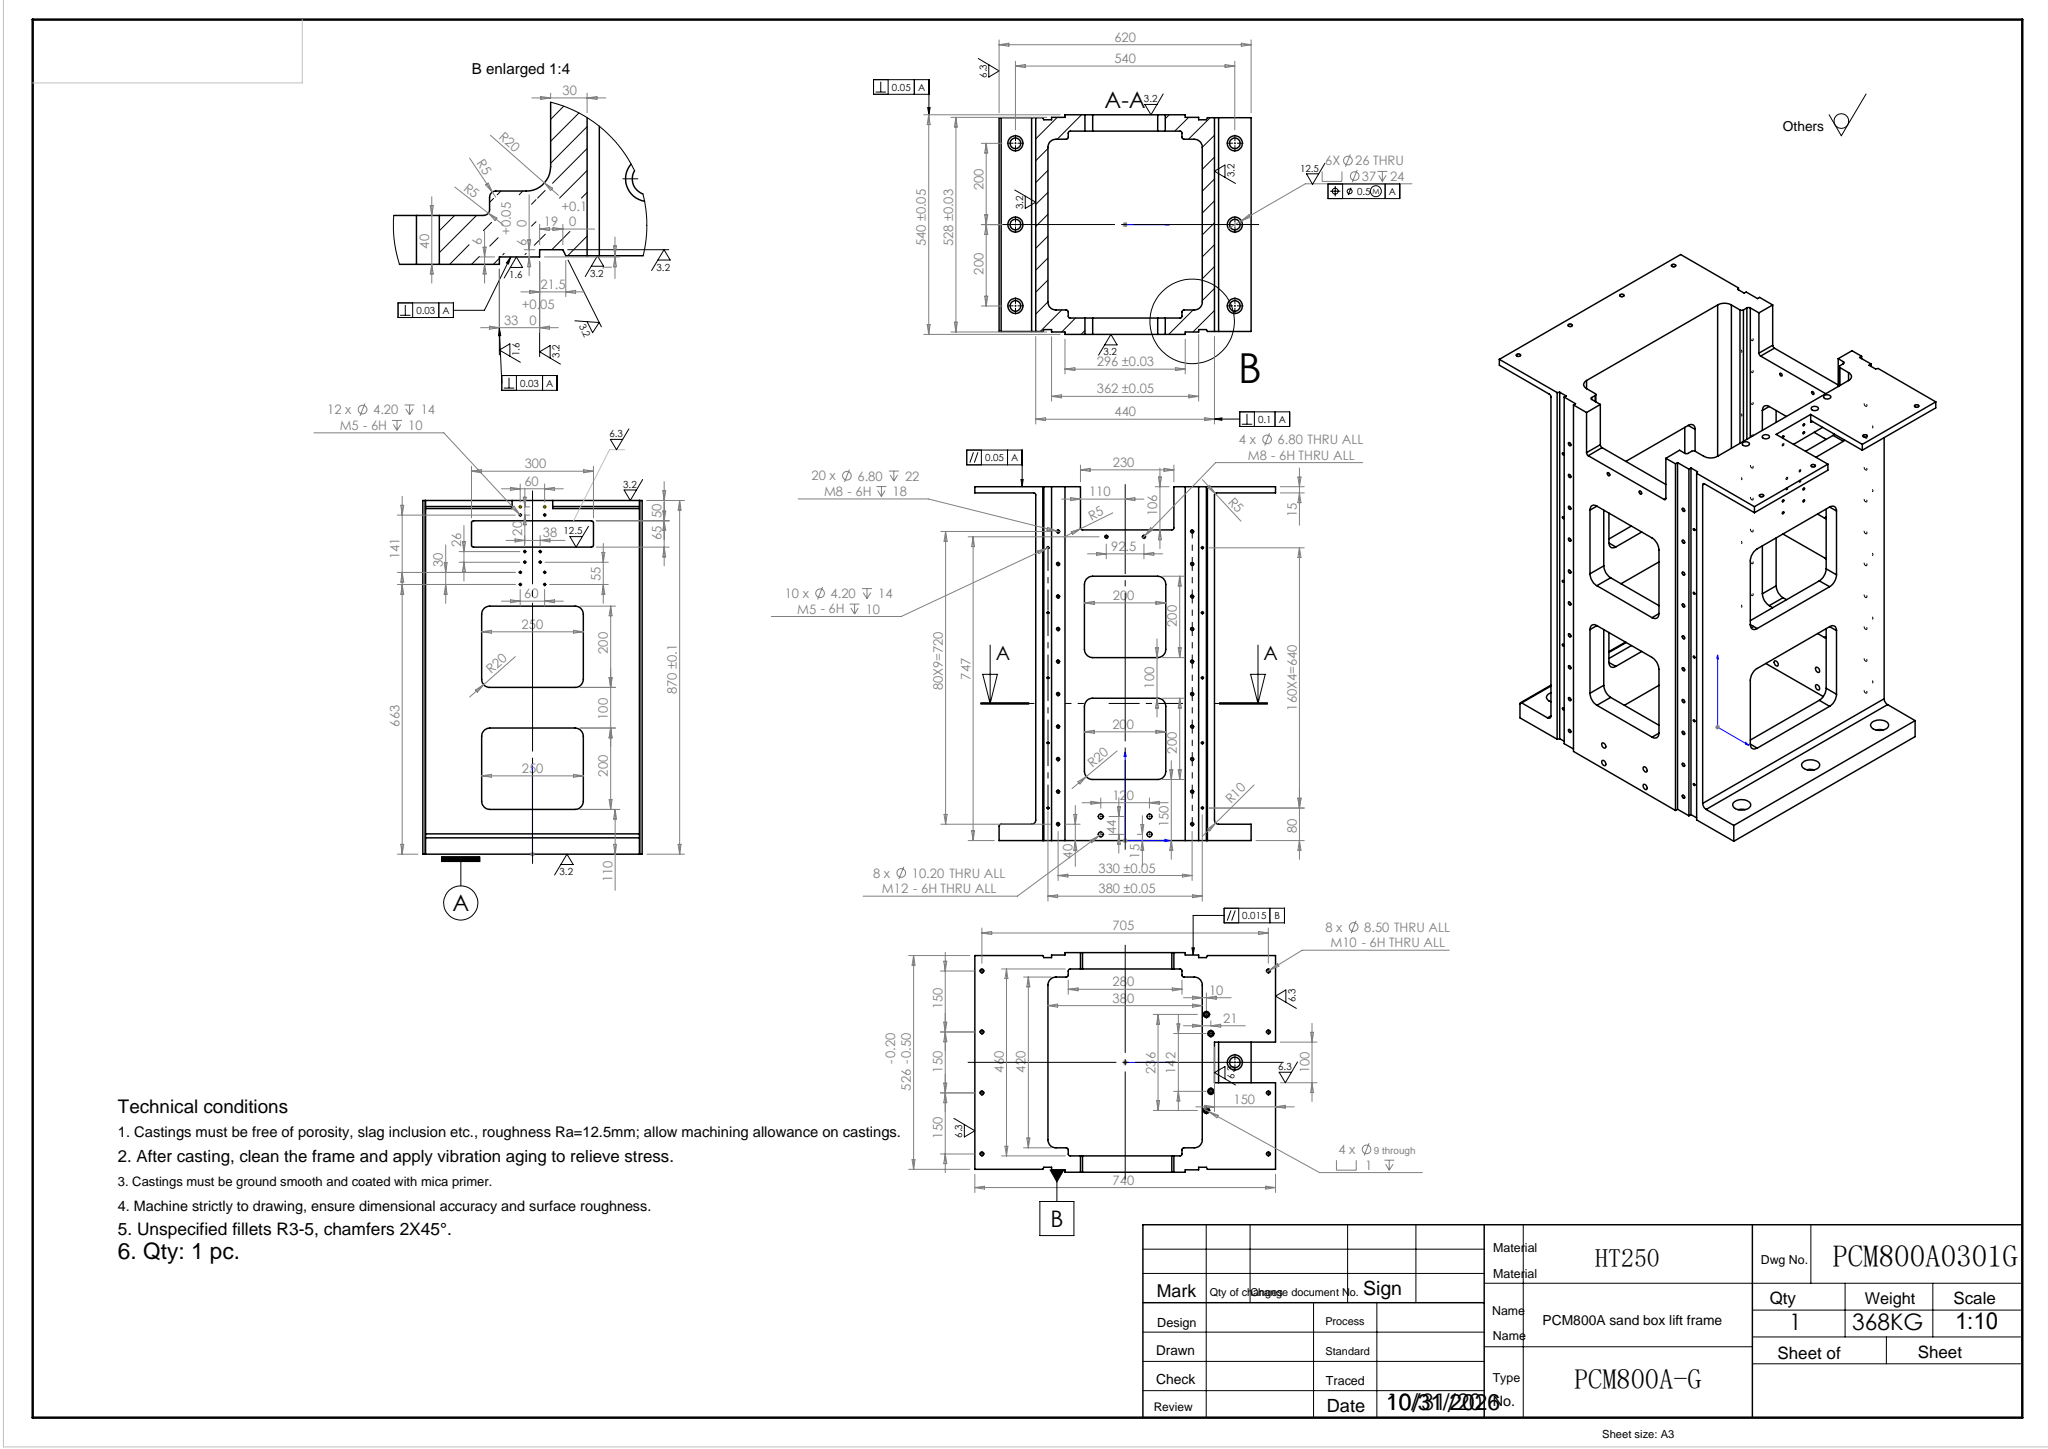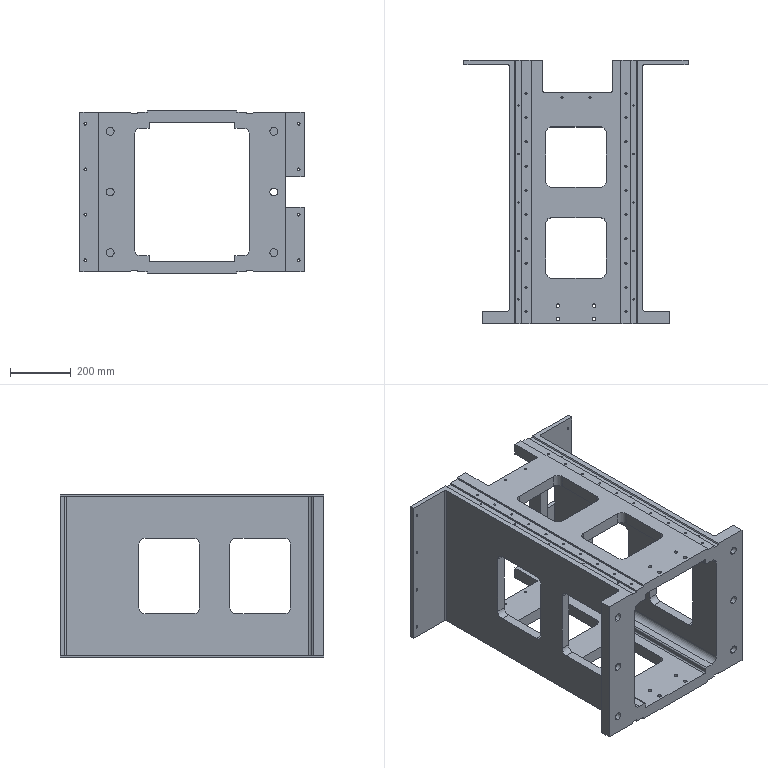Part | SolidWorks | features HoleWzd 9, 3DProfileFeature 8, MirrorPattern 7, Cut 5, Fillet 5, Boss 2, LPattern 2, Extrusion 1 | 1 solid | 533 faces | box 740 x 870 x 540 mm | volume 47222068 mm3 | cylinder 282 | cone 144 | plane 107 | commonest cylinder face diameters 6.8 x88 4.2 x64 40 x36 10 x20 8.5 x16 12 x16